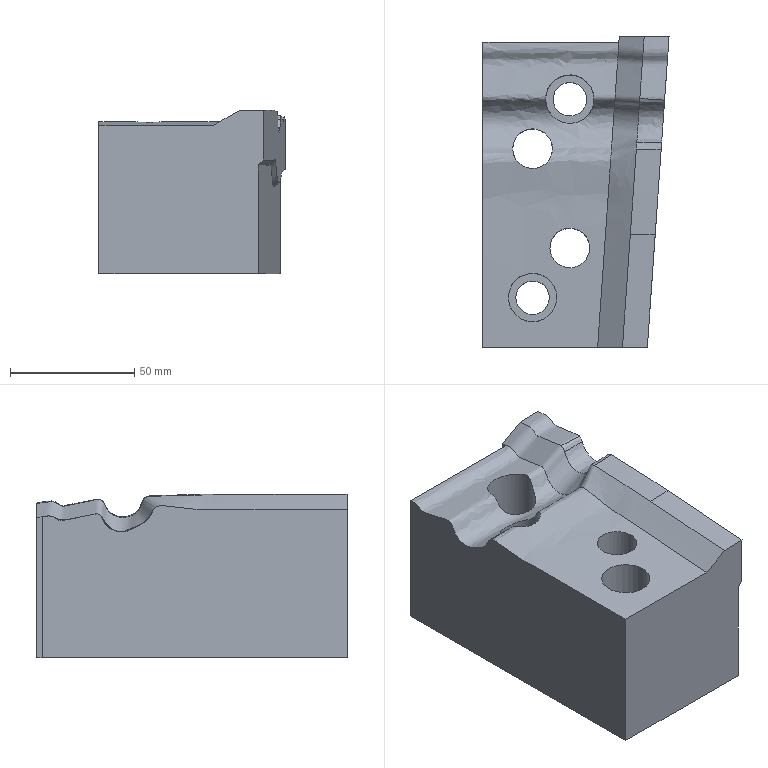Part | NX | features solid 2 | 1 solid | 25 faces | box 75 x 125.871 x 65.967 mm | volume 453452 mm3 | spline 10 | plane 9 | cylinder 6 | commonest cylinder face diameters 13.5 x2 16 x2 19.5 x2